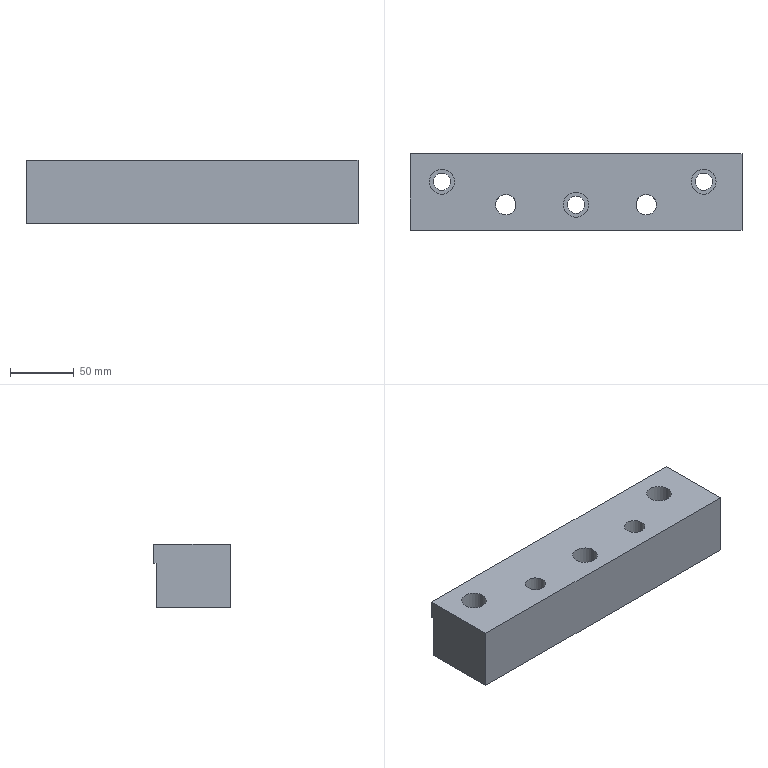Part | NX | features solid 2 | 1 solid | 20 faces | box 260 x 60 x 50 mm | volume 708560 mm3 | cylinder 8 | plane 7 | spline 5 | commonest cylinder face diameters 13.5 x3 19.5 x3 16 x2